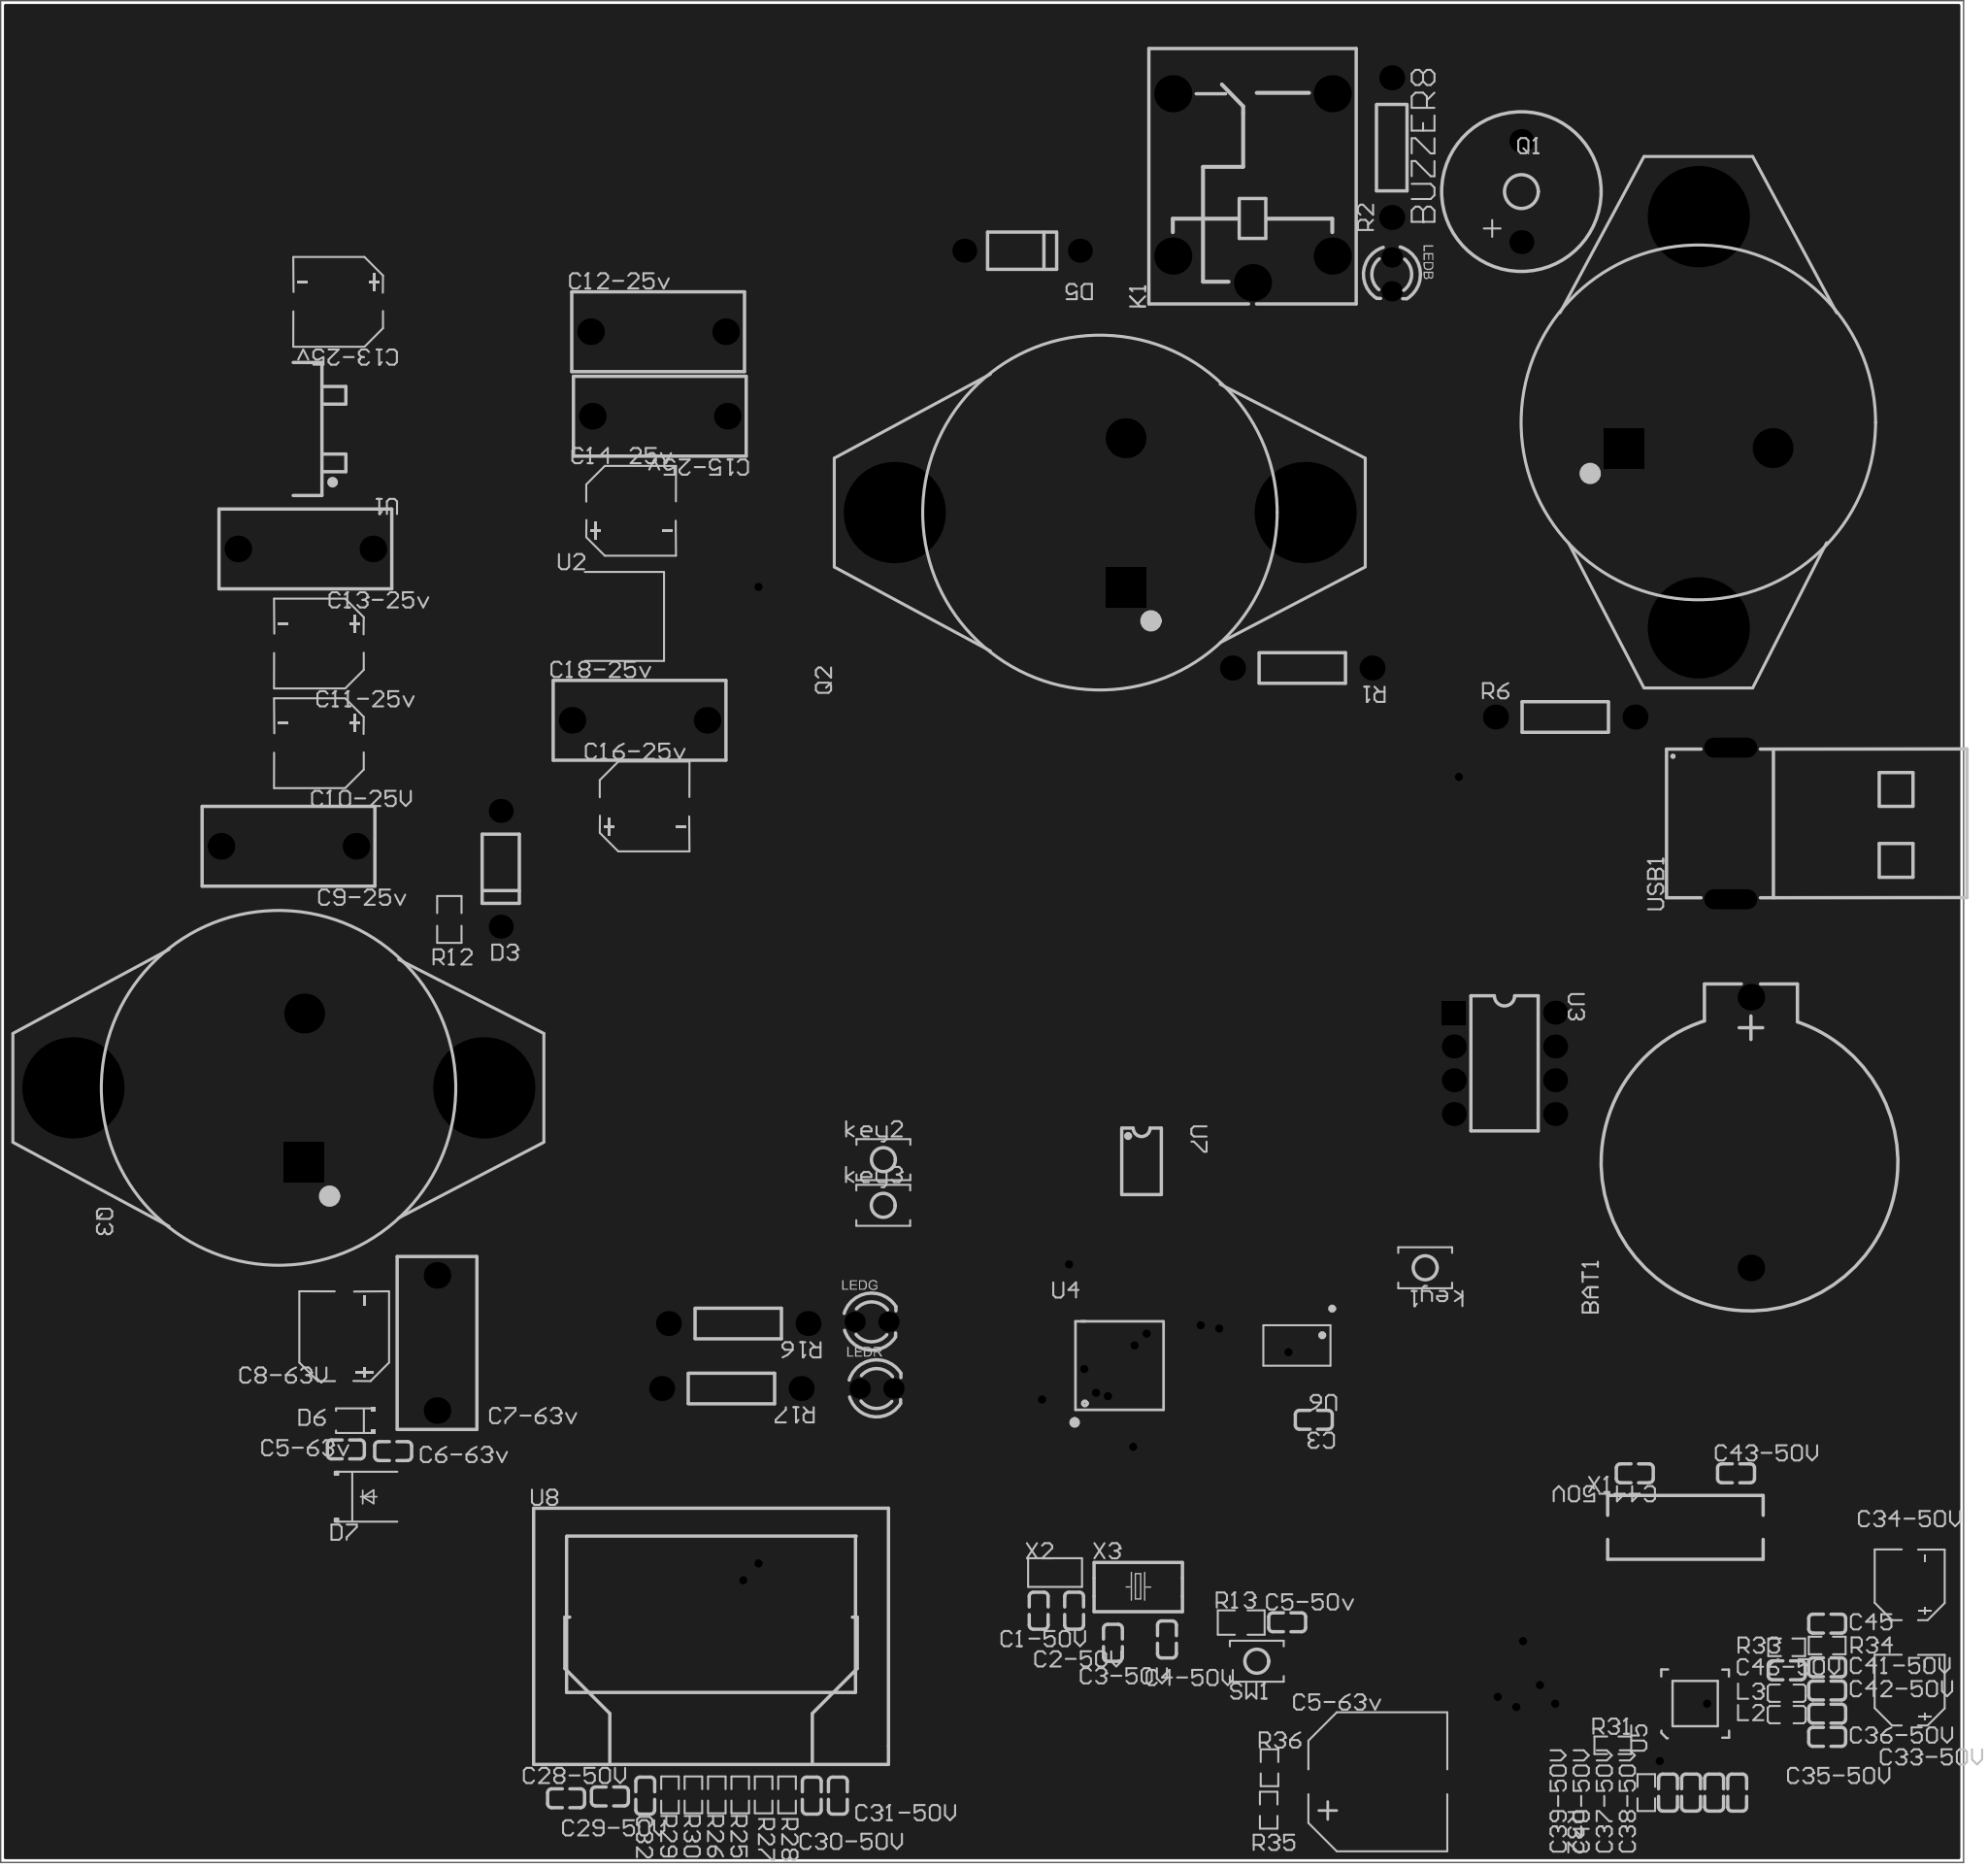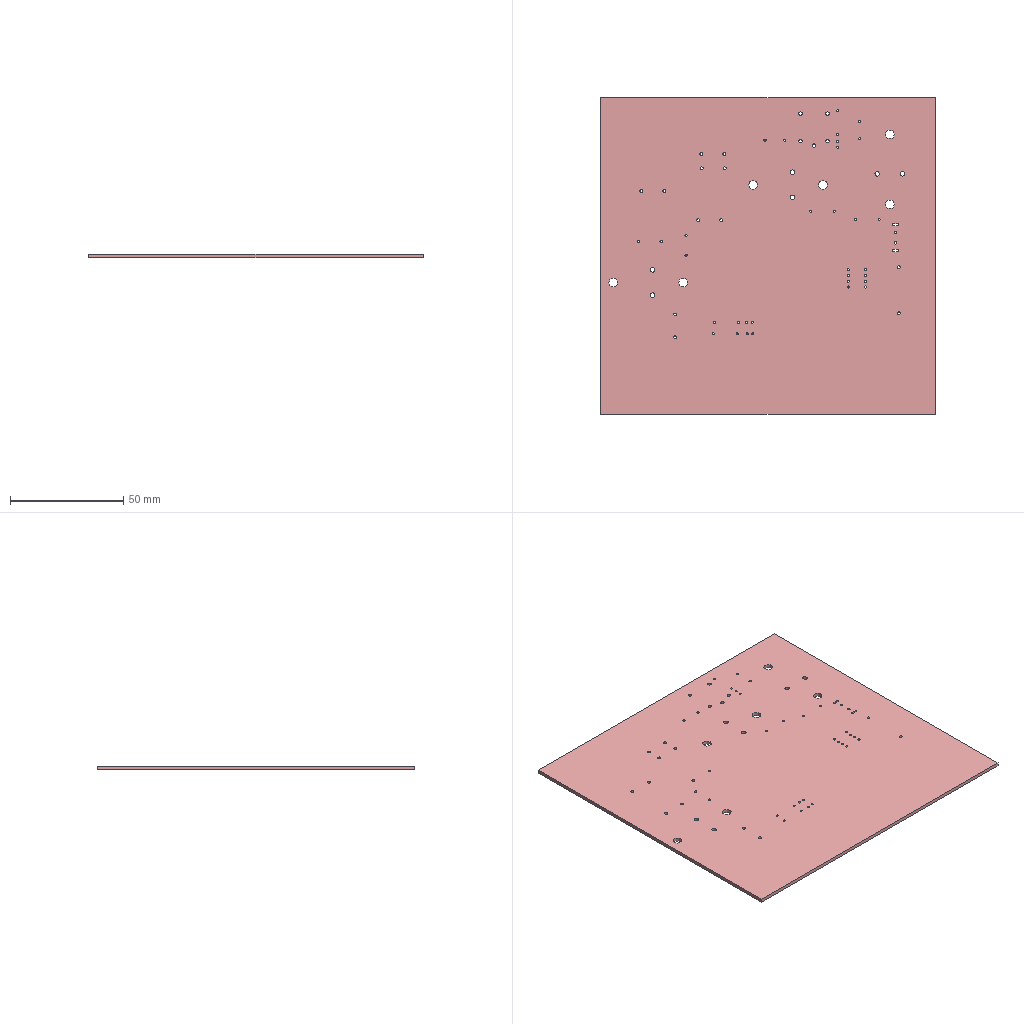Circuit board layout | Altium Designer | box 147.7 x 140 x 1.6 mm
Layer stack:
# Altium Designer layer stack of  (unit mm; dielectric type: 0 none, 1 core, 2 prepreg, 3 surface material)
index,name,kind,layer,copper_thickness_mm,dielectric_type,dielectric_thickness_mm,dielectric_material,dielectric_constant
0,Top Paste Mask Layer,other,,,,,,
1,Top Silkscreen Layer,other,,,,,,
2,Top Solder Mask Layer,dielectric,,,3,0.01,,3.3
3,Top Layer,copper,Top Layer,0.035,,,,
4,Dielectric1,dielectric,,,3,1.51,FR4,4.5
5,Bottom Layer,copper,Bottom Layer,0.035,,,,
6,Bottom Solder Mask Layer,dielectric,,,3,0.01,,3.3
7,Bottom Silkscreen Layer,other,,,,,,
8,Bottom Paste Mask Layer,other,,,,,,
# drill layer pairs: low layer,high layer
drill_pair,Top Layer,Bottom Layer
Part placement:
Designator,Comment,Layer,Footprint,Center-X(mm),Center-Y(mm),Rotation
BAT1,CR2032-2-1,TopLayer,BAT-TH_CR2032-2-1,217.043,140.081,90
BUZZER8,buzzer-12X9,TopLayer,BUZ-TH_BD12.0-P7.60-D0.6-FD,199.771,210.82,90
C1-50V,22pF,TopLayer,C0603,163.449,104.14,270
C2-50V,22pF,TopLayer,C0603,166.116,104.14,270
C3-50V,22pF,TopLayer,C0603,169.037,101.727,270
C4-50V,22pF,TopLayer,C0603,173.101,101.981,270
C5-50v,100nF,TopLayer,C0603,182.148,103.272,0
C10-25V,100uF,TopLayer,CAP-SMD_BD6.3-L6.6-W6.6-LS7.3-FD-H7.7,109.287,169.353,180
C11-25v,100uF,TopLayer,CAP-SMD_BD6.3-L6.6-W6.6-LS7.3-FD-H7.7,109.287,176.846,180
C13-25v,100uF,TopLayer,CAP-SMD_BD6.3-L6.6-W6.6-LS7.3-FD-H7.7,110.736,202.53,180
D3,1N4742A,TopLayer,DO-41_BD2.4-L4.7-P8.70-D0.9-RD,122.972,159.915,90
D6,1N4003W,TopLayer,SOD-123FL_L2.7-W1.8-LS3.8-RD,111.954,118.426,180
D7,SMBJ51A,TopLayer,SMB_L4.3-W3.6-LS5.4-R-RD,112.971,112.711,0
K1,,TopLayer,RELAY-TH_SRD-DCXXV-SL-C,179.541,211.075,90
LEDB,,TopLayer,LED_TH-3mm,190.016,204.598,270
Q3,2N3055,TopLayer,TO-3_L39.4-W26.7-P10.92-BL,106.24,143.445,90
R1,,TopLayer,RES-TH_BD2.3-L6.5-P10.50-D0.5,183.285,175.007,180
R2,,TopLayer,RES-TH_BD2.3-L6.5-P10.50-D0.5,190.016,214.123,90
R6,,TopLayer,RES-TH_BD2.3-L6.5-P10.50-D0.5,203.073,171.323,0
R12,10kΩ,TopLayer,R0805,119.105,156.105,90
R13,10kΩ,TopLayer,R0805,178.689,103.251,0
SW1,TS-1088-AR02016,TopLayer,SW-SMD_L3.9-W3.0-P4.45,179.862,100.344,0
U1,L7805ABD2T-TR,TopLayer,TO-263-2_L10.0-W9.2-P5.08-LS15.3-TL-CW,108.017,192.975,180
U3,DS1302,TopLayer,DIP-8_L9.7-W6.4-P2.54-LS7.6-BL,198.501,145.288,270
U2,LD1117DT33TR,TopLayer,TO-252-2_L6.6-W6.1-P4.57-LS9.9-BR-CW,133.876,178.883,0
U4,STM32F103C8T6,TopLayer,LQFP-48_L7.0-W7.0-P0.50-LS9.0-BL,169.545,122.555,0
X2,32.768kHz,TopLayer,CRYSTAL-SMD_L3.2-W1.5-1,164.683,107.009,180
X3,8MHz,TopLayer,CRYSTAL-SMD_L5.0-W3.2,170.942,105.918,180
C5-63v,100uF,TopLayer,CAP-SMD_BD10.0-L10.3-W10.3-LS11.0-FD_1,188.97,91.28,0
D5,1N4003-E3/54,TopLayer,DO-41_BD2.4-L4.7-P8.70-D0.9-RD,162.203,206.376,180
key1,TS-1088-AR02016,TopLayer,SW-SMD_L3.9-W3.0-P4.45,192.532,129.921,180
key2,TS-1088-AR02016,TopLayer,SW-SMD_L3.9-W3.0-P4.45,151.765,138.049,0
key3,TS-1088-AR02016,TopLayer,SW-SMD_L3.9-W3.0-P4.45,151.755,134.615,0
LEDG,,TopLayer,LED_TH-3mm,150.876,125.857,0
Q2,2N3055,TopLayer,TO-3_L39.4-W26.7-P10.92-BL,168.045,186.691,90
R16,,TopLayer,RES-TH_BD2.3-L6.5-P10.50-D0.5,140.843,125.73,180
C5-63v,100nF,TopLayer,C0603,111.32,116.267,180
C6-63v,100nF,TopLayer,C0603,114.876,116.14,180
C7-63v,100nF,TopLayer,CAP-TH_L13.0-W6.0-P10.00-D1.0,118.177,124.268,90
C8-63V,100uF,TopLayer,CAP-SMD_BD6.3-L6.6-W6.6-LS7.3-FD-H7.7,111.192,124.776,90
C9-25v,100nF,TopLayer,CAP-TH_L13.0-W6.0-P10.00-D1.0,107.001,161.606,180
C12-25v,100nF,TopLayer,CAP-TH_L13.0-W6.0-P10.00-D1.0,134.815,200.285,0
C13-25v,100nF,TopLayer,CAP-TH_L13.0-W6.0-P10.00-D1.0,108.272,183.958,180
C14-25v,100uF,TopLayer,CAP-SMD_BD6.3-L6.6-W6.6-LS7.3-FD-H7.7,132.782,186.823,0
C15-25v,100nF,TopLayer,CAP-TH_L13.0-W6.0-P10.00-D1.0,134.941,193.935,180
C16-25v,100uF,TopLayer,CAP-SMD_BD6.3-L6.6-W6.6-LS7.3-FD-H7.7,133.798,164.598,0
C18-25v,100nF,TopLayer,CAP-TH_L13.0-W6.0-P10.00-D1.0,133.417,171.075,0
C28-50V,1uF,TopLayer,C0603,127.889,90.043,180
C29-50V,1uF,TopLayer,C0603,131.186,90.179,180
C30-50V,4.7uF,TopLayer,C0603,146.376,90.241,90
C31-50V,2.2uF,TopLayer,C0603,148.338,90.241,90
C32,10uF,TopLayer,C0603,133.845,90.241,90
C33-50V,0.1uF,TopLayer,CAP-SMD_BD5.0-L5.3-W5.3-FD,229.002,98.173,90
C34-50V,0.1uF,TopLayer,CAP-SMD_BD5.0-L5.3-W5.3-FD,229.004,106.089,90
C35-50V,47pF,TopLayer,C0603,222.781,96.401,180
C36-50V,15pF,TopLayer,C0603,222.781,94.659,0
C37-50V,180pF,TopLayer,C0603,214.274,90.468,90
C38-50V,10pF,TopLayer,C0603,216.008,90.468,90
C39-50V,180pF,TopLayer,C0603,210.804,90.468,90
C40-50V,10pF,TopLayer,C0603,212.539,90.468,90
C41-50V,15pF,TopLayer,C0603,222.781,99.885,0
C42-50V,47pF,TopLayer,C0603,222.781,98.143,0
C43-50V,15pF,TopLayer,C0603,215.923,114.471,0
C44-50V,15pF,TopLayer,C0603,208.303,114.471,180
C45,0.1uF,TopLayer,C0603,222.781,103.168,0
C46-50V,0.1uF,TopLayer,C0603,219.733,99.66,0
L2,2.2uH,TopLayer,L0603,219.733,96.33,0
L3,2.2uH,TopLayer,L0603,219.733,97.94,0
R25,4.7K,TopLayer,R0603,140.991,90.297,270
R26,4.7K,TopLayer,R0603,139.23,90.297,270
R27,0,TopLayer,R0603,142.753,90.297,90
R28,910K,TopLayer,R0603,144.514,90.297,90
R29,10K,TopLayer,R0603,135.707,90.297,270
R30,10K,TopLayer,R0603,137.468,90.297,270
R31,1K,TopLayer,R0603,206.652,94.024,0
R32,10k,TopLayer,R0603,209.169,90.468,270
R33,820Ω,TopLayer,R0603,219.733,101.39,0
R34,5.1k,TopLayer,R0603,222.781,101.526,0
R36,1kΩ,TopLayer,R0603,180.818,92.338,270
U8,X096-2864KLBAG01-H30,TopLayer,OLED-SMD_X096-2864KLBAG01-H30,138.797,102.386,0
U5,MFRC522,TopLayer,QFN32,212.848,97.161,90
X1,27.12MHz,TopLayer,OSC-SMD_L11.4-W4.5-LS12.5,212.113,110.407,0
C3,100nF,TopLayer,C0603,184.15,118.491,180
LEDR,,TopLayer,LED_TH-3mm,151.252,120.843,0
Q1,2N3055,TopLayer,TO-3_L39.4-W26.7-P10.92-BL,213.086,193.482,0
R17,,TopLayer,RES-TH_BD2.3-L6.5-P10.50-D0.5,140.33,120.844,180
R35,30kΩ,TopLayer,R0603,180.756,89.145,90
U6,AT24C02,TopLayer,SOIC-8_L4.9-W3.9-P1.27-LS6.0-BL,182.88,124.079,180
U7,CH340N,TopLayer,SOP-8_L4.9-W3.9-P1.27-LS6.0-BL,171.196,137.922,270
USB1,U217-041N-4BV81,TopLayer,USB-A-SMD_U217-041N-4BV81,214.122,163.322,90
Pad and via stacks:
# Altium Designer via and pad stacks of  (unit mm). Each distinct definition once, with the count of objects using it.
# via: kind,start_layer,end_layer,hole_mm,diameter_mm,mode(0 simple;1 top-mid-bottom;2 full stack),diameter_per_layer,count,example_net
# pad: kind,layer,hole_mm,hole_type(0 round;1 square;2 slot),plating,top_size,top_shape(1 round;2 rect;3 octagon;9 rounded rect),mid_size,bottom_size,mode,footprint,size_per_layer,count,example
pad,Multi-Layer,1.2,0,plated,2x2,1,2x2,2x2,0,BAT-TH_CR2032-2-1,,2,BAT1.2
pad,Multi-Layer,1.001,0,plated,1.801x1.801,1,1.801x1.801,1.801x1.801,0,BUZ-TH_BD12.0-P7.60-D0.6-FD,,2,BUZZER8.1
pad,Multi-Layer,1,0,plated,1.8x1.8,1,1.8x1.8,1.8x1.8,0,DO-41_BD2.4-L4.7-P8.70-D0.9-RD,,4,D3.1
pad,Multi-Layer,1.524,0,plated,2.794x2.794,1,2.794x2.794,2.794x2.794,0,RELAY-TH_SRD-DCXXV-SL-C,,5,K1.2
pad,Multi-Layer,0.9144,0,plated,1.524x1.524,1,1.524x1.524,1.524x1.524,0,LED_TH-3mm,,6,LEDB.1
pad,Multi-Layer,2,0,plated,3x3,2,3x3,3x3,0,TO-3_L39.4-W26.7-P10.92-BL,,3,Q3.1
pad,Multi-Layer,2,0,plated,3x3,1,3x3,3x3,0,TO-3_L39.4-W26.7-P10.92-BL,,3,Q3.2
pad,Multi-Layer,3.81,0,plated,7.62x7.62,1,7.62x7.62,7.62x7.62,0,TO-3_L39.4-W26.7-P10.92-BL,,6,Q3.3
pad,Multi-Layer,0.8992,0,plated,1.88x1.88,1,1.88x1.88,1.88x1.88,0,RES-TH_BD2.3-L6.5-P10.50-D0.5,,10,R1.1
pad,Multi-Layer,1,0,plated,1.8x1.8,2,1.8x1.8,1.8x1.8,0,DIP-8_L9.7-W6.4-P2.54-LS7.6-BL,,1,U3.1
pad,Multi-Layer,1,0,plated,1.8x1.8,1,1.8x1.8,1.8x1.8,0,DIP-8_L9.7-W6.4-P2.54-LS7.6-BL,,7,U3.2
pad,Multi-Layer,1.3,0,plated,2x2,1,2x2,2x2,0,CAP-TH_L13.0-W6.0-P10.00-D1.0,,12,C7-63v.1
pad,Multi-Layer,1.001,2,plated,1.501x4,1,1.501x4,1.501x4,0,USB-A-SMD_U217-041N-4BV81,,2,USB1.5
pad,Top Layer,0,0,plated,0.8x0.9,2,0.8x0.9,0.8x0.9,0,C0603,,50,C1-50V.2
pad,Top Layer,0,0,plated,3.5x1.2,2,3.5x1.2,3.5x1.2,0,CAP-SMD_BD6.3-L6.6-W6.6-LS7.3-FD-H7.7,,12,C10-25V.1
pad,Top Layer,0,0,plated,1.2x1.2,2,1.2x1.2,1.2x1.2,0,SOD-123FL_L2.7-W1.8-LS3.8-RD,,2,D6.2
pad,Top Layer,0,0,plated,1.96x2.94,2,1.96x2.94,1.96x2.94,0,SMB_L4.3-W3.6-LS5.4-R-RD,,2,D7.1
pad,Top Layer,0,0,plated,1.133x1.377,2,1.133x1.377,1.133x1.377,0,R0805,,4,R12.2
pad,Top Layer,0,0,plated,1.23x1.86,2,1.23x1.86,1.23x1.86,0,SW-SMD_L3.9-W3.0-P4.45,,8,SW1.1
pad,Top Layer,0,0,plated,9x10.2,2,9x10.2,9x10.2,0,TO-263-2_L10.0-W9.2-P5.08-LS15.3-TL-CW,,1,U1.2
pad,Top Layer,0,0,plated,3.5x1.6,2,3.5x1.6,3.5x1.6,0,TO-263-2_L10.0-W9.2-P5.08-LS15.3-TL-CW,,2,U1.3
pad,Top Layer,0,0,plated,3x1.6,2,3x1.6,3x1.6,0,TO-252-2_L6.6-W6.1-P4.57-LS9.9-BR-CW,,2,U2.1
pad,Top Layer,0,0,plated,6.2x5.8,2,6.2x5.8,6.2x5.8,0,TO-252-2_L6.6-W6.1-P4.57-LS9.9-BR-CW,,1,U2.2
pad,Top Layer,0,0,plated,0.27x1.5,1,0.27x1.5,0.27x1.5,0,LQFP-48_L7.0-W7.0-P0.50-LS9.0-BL,,24,U4.1
pad,Top Layer,0,0,plated,1.5x0.27,1,1.5x0.27,1.5x0.27,0,LQFP-48_L7.0-W7.0-P0.50-LS9.0-BL,,24,U4.13
pad,Top Layer,0,0,plated,1.05x1.7,2,1.05x1.7,1.05x1.7,0,CRYSTAL-SMD_L3.2-W1.5-1,,2,X2.2
pad,Top Layer,0,0,plated,1.9x2.4,2,1.9x2.4,1.9x2.4,0,CRYSTAL-SMD_L5.0-W3.2,,2,X3.2
pad,Top Layer,0,0,plated,4.2x1.5,2,4.2x1.5,4.2x1.5,0,CAP-SMD_BD10.0-L10.3-W10.3-LS11.0-FD_1,,2,C5-63v.1
pad,Top Layer,0,0,plated,2.8x1.1,2,2.8x1.1,2.8x1.1,0,CAP-SMD_BD5.0-L5.3-W5.3-FD,,4,C33-50V.1
pad,Top Layer,0,0,plated,0.8x0.864,2,0.8x0.864,0.8x0.864,0,L0603,,4,L2.1
pad,Top Layer,0,0,plated,0.8065x0.864,2,0.8065x0.864,0.8065x0.864,0,R0603,,24,R25.2
pad,Top Layer,0,0,plated,0.5x4,2,0.5x4,0.5x4,0,OLED-SMD_X096-2864KLBAG01-H30,,30,U8.1
pad,Top Layer,0,0,plated,1.524x0.3302,1,1.524x0.3302,1.524x0.3302,0,QFN32,,32,U5.26
pad,Top Layer,0,0,plated,5.5x2,2,5.5x2,5.5x2,0,OSC-SMD_L11.4-W4.5-LS12.5,,2,X1.1
pad,Top Layer,0,0,plated,0.588x2.045,1,0.588x2.045,0.588x2.045,0,SOIC-8_L4.9-W3.9-P1.27-LS6.0-BL,,8,U6.5
pad,Top Layer,0,0,plated,0.63x1.865,1,0.63x1.865,0.63x1.865,0,SOP-8_L4.9-W3.9-P1.27-LS6.0-BL,,8,U7.1
pad,Top Layer,0,0,plated,1.199x2.499,2,1.199x2.499,1.199x2.499,0,USB-A-SMD_U217-041N-4BV81,,4,USB1.1
via,Top Layer,Bottom Layer,0.3048,0.61,0,,22,SCK
Copper pours:
name,layer,net,type(0 solid;1 hatched;2 none)
Top Layer-GND,Top Layer,GND,0
Bottom Layer-GND,Bottom Layer,GND,0